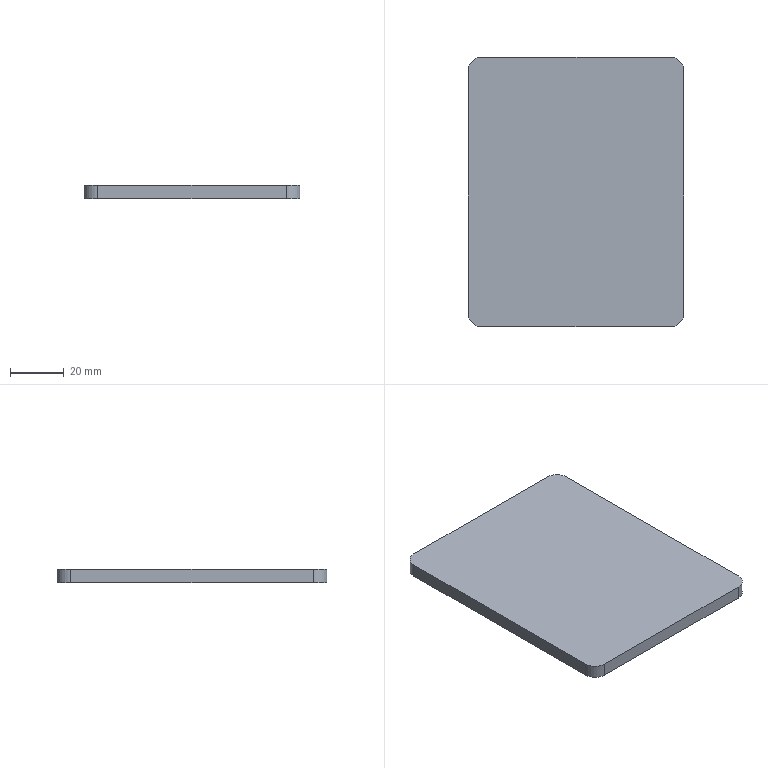Part | SolidWorks | features Extrusion 1, Fillet 1 | 1 solid | 10 faces | box 80 x 100 x 5 mm | volume 39893 mm3 | plane 6 | cylinder 4 | commonest cylinder face diameters 10 x4
STEP:
#1=CARTESIAN_POINT('',(0.,-5.,0.));
#2=VERTEX_POINT('',#1);
#3=CARTESIAN_POINT('',(0.,-95.,0.));
#4=VERTEX_POINT('',#3);
#5=CARTESIAN_POINT('',(0.,0.,0.));
#6=DIRECTION('',(0.,-1.,0.));
#7=VECTOR('',#6,1000.);
#8=LINE('',#5,#7);
#9=EDGE_CURVE('',#2,#4,#8,.T.);
#10=ORIENTED_EDGE('',*,*,#9,.T.);
#11=CARTESIAN_POINT('',(0.,-95.,5.));
#12=VERTEX_POINT('',#11);
#13=CARTESIAN_POINT('',(0.,-95.,5.));
#14=DIRECTION('',(0.,0.,1.));
#15=VECTOR('',#14,1000.);
#16=LINE('',#13,#15);
#17=EDGE_CURVE('',#4,#12,#16,.T.);
#18=ORIENTED_EDGE('',*,*,#17,.T.);
#19=CARTESIAN_POINT('',(0.,-5.,5.));
#20=VERTEX_POINT('',#19);
#21=CARTESIAN_POINT('',(0.,0.,5.));
#22=DIRECTION('',(0.,-1.,0.));
#23=VECTOR('',#22,1000.);
#24=LINE('',#21,#23);
#25=EDGE_CURVE('',#20,#12,#24,.T.);
#26=ORIENTED_EDGE('',*,*,#25,.F.);
#27=CARTESIAN_POINT('',(0.,-5.,5.));
#28=DIRECTION('',(0.,0.,-1.));
#29=VECTOR('',#28,1000.);
#30=LINE('',#27,#29);
#31=EDGE_CURVE('',#20,#2,#30,.T.);
#32=ORIENTED_EDGE('',*,*,#31,.T.);
#33=EDGE_LOOP('',(#10,#18,#26,#32));
#34=FACE_OUTER_BOUND('',#33,.T.);
#35=CARTESIAN_POINT('',(0.,0.,5.));
#36=DIRECTION('',(1.,0.,0.));
#37=DIRECTION('',(0.,1.,0.));
#38=AXIS2_PLACEMENT_3D('',#35,#36,#37);
#39=PLANE('',#38);
#40=ADVANCED_FACE('',(#34),#39,.F.);
#41=CARTESIAN_POINT('',(5.,-100.,0.));
#42=VERTEX_POINT('',#41);
#43=CARTESIAN_POINT('',(75.,-100.,0.));
#44=VERTEX_POINT('',#43);
#45=CARTESIAN_POINT('',(0.,-100.,0.));
#46=DIRECTION('',(1.,0.,0.));
#47=VECTOR('',#46,1000.);
#48=LINE('',#45,#47);
#49=EDGE_CURVE('',#42,#44,#48,.T.);
#50=ORIENTED_EDGE('',*,*,#49,.T.);
#51=CARTESIAN_POINT('',(75.,-100.,5.));
#52=VERTEX_POINT('',#51);
#53=CARTESIAN_POINT('',(75.,-100.,5.));
#54=DIRECTION('',(0.,0.,1.));
#55=VECTOR('',#54,1000.);
#56=LINE('',#53,#55);
#57=EDGE_CURVE('',#44,#52,#56,.T.);
#58=ORIENTED_EDGE('',*,*,#57,.T.);
#59=CARTESIAN_POINT('',(5.,-100.,5.));
#60=VERTEX_POINT('',#59);
#61=CARTESIAN_POINT('',(0.,-100.,5.));
#62=DIRECTION('',(1.,0.,0.));
#63=VECTOR('',#62,1000.);
#64=LINE('',#61,#63);
#65=EDGE_CURVE('',#60,#52,#64,.T.);
#66=ORIENTED_EDGE('',*,*,#65,.F.);
#67=CARTESIAN_POINT('',(5.,-100.,5.));
#68=DIRECTION('',(0.,0.,-1.));
#69=VECTOR('',#68,1000.);
#70=LINE('',#67,#69);
#71=EDGE_CURVE('',#60,#42,#70,.T.);
#72=ORIENTED_EDGE('',*,*,#71,.T.);
#73=EDGE_LOOP('',(#50,#58,#66,#72));
#74=FACE_OUTER_BOUND('',#73,.T.);
#75=CARTESIAN_POINT('',(0.,-100.,5.));
#76=DIRECTION('',(0.,1.,0.));
#77=DIRECTION('',(0.,0.,1.));
#78=AXIS2_PLACEMENT_3D('',#75,#76,#77);
#79=PLANE('',#78);
#80=ADVANCED_FACE('',(#74),#79,.F.);
#81=CARTESIAN_POINT('',(80.,-95.,5.));
#82=VERTEX_POINT('',#81);
#83=CARTESIAN_POINT('',(80.,-5.,5.));
#84=VERTEX_POINT('',#83);
#85=CARTESIAN_POINT('',(80.,0.,5.));
#86=DIRECTION('',(0.,1.,0.));
#87=VECTOR('',#86,1000.);
#88=LINE('',#85,#87);
#89=EDGE_CURVE('',#82,#84,#88,.T.);
#90=ORIENTED_EDGE('',*,*,#89,.F.);
#91=CARTESIAN_POINT('',(80.,-95.,0.));
#92=VERTEX_POINT('',#91);
#93=CARTESIAN_POINT('',(80.,-95.,5.));
#94=DIRECTION('',(0.,0.,-1.));
#95=VECTOR('',#94,1000.);
#96=LINE('',#93,#95);
#97=EDGE_CURVE('',#82,#92,#96,.T.);
#98=ORIENTED_EDGE('',*,*,#97,.T.);
#99=CARTESIAN_POINT('',(80.,-5.,0.));
#100=VERTEX_POINT('',#99);
#101=CARTESIAN_POINT('',(80.,0.,0.));
#102=DIRECTION('',(0.,1.,0.));
#103=VECTOR('',#102,1000.);
#104=LINE('',#101,#103);
#105=EDGE_CURVE('',#92,#100,#104,.T.);
#106=ORIENTED_EDGE('',*,*,#105,.T.);
#107=CARTESIAN_POINT('',(80.,-5.,5.));
#108=DIRECTION('',(0.,0.,1.));
#109=VECTOR('',#108,1000.);
#110=LINE('',#107,#109);
#111=EDGE_CURVE('',#100,#84,#110,.T.);
#112=ORIENTED_EDGE('',*,*,#111,.T.);
#113=EDGE_LOOP('',(#90,#98,#106,#112));
#114=FACE_OUTER_BOUND('',#113,.T.);
#115=CARTESIAN_POINT('',(80.,0.,5.));
#116=DIRECTION('',(-1.,0.,0.));
#117=DIRECTION('',(0.,-1.,0.));
#118=AXIS2_PLACEMENT_3D('',#115,#116,#117);
#119=PLANE('',#118);
#120=ADVANCED_FACE('',(#114),#119,.F.);
#121=CARTESIAN_POINT('',(75.,0.,5.));
#122=VERTEX_POINT('',#121);
#123=CARTESIAN_POINT('',(5.,0.,5.));
#124=VERTEX_POINT('',#123);
#125=CARTESIAN_POINT('',(0.,0.,5.));
#126=DIRECTION('',(-1.,0.,0.));
#127=VECTOR('',#126,1000.);
#128=LINE('',#125,#127);
#129=EDGE_CURVE('',#122,#124,#128,.T.);
#130=ORIENTED_EDGE('',*,*,#129,.F.);
#131=CARTESIAN_POINT('',(75.,0.,0.));
#132=VERTEX_POINT('',#131);
#133=CARTESIAN_POINT('',(75.,0.,5.));
#134=DIRECTION('',(0.,0.,-1.));
#135=VECTOR('',#134,1000.);
#136=LINE('',#133,#135);
#137=EDGE_CURVE('',#122,#132,#136,.T.);
#138=ORIENTED_EDGE('',*,*,#137,.T.);
#139=CARTESIAN_POINT('',(5.,0.,0.));
#140=VERTEX_POINT('',#139);
#141=CARTESIAN_POINT('',(0.,0.,0.));
#142=DIRECTION('',(-1.,0.,0.));
#143=VECTOR('',#142,1000.);
#144=LINE('',#141,#143);
#145=EDGE_CURVE('',#132,#140,#144,.T.);
#146=ORIENTED_EDGE('',*,*,#145,.T.);
#147=CARTESIAN_POINT('',(5.,0.,5.));
#148=DIRECTION('',(0.,0.,1.));
#149=VECTOR('',#148,1000.);
#150=LINE('',#147,#149);
#151=EDGE_CURVE('',#140,#124,#150,.T.);
#152=ORIENTED_EDGE('',*,*,#151,.T.);
#153=EDGE_LOOP('',(#130,#138,#146,#152));
#154=FACE_OUTER_BOUND('',#153,.T.);
#155=CARTESIAN_POINT('',(0.,0.,5.));
#156=DIRECTION('',(0.,-1.,0.));
#157=DIRECTION('',(0.,0.,-1.));
#158=AXIS2_PLACEMENT_3D('',#155,#156,#157);
#159=PLANE('',#158);
#160=ADVANCED_FACE('',(#154),#159,.F.);
#161=ORIENTED_EDGE('',*,*,#65,.T.);
#162=CARTESIAN_POINT('',(75.,-95.,5.));
#163=DIRECTION('',(0.,0.,1.));
#164=DIRECTION('',(1.,0.,0.));
#165=AXIS2_PLACEMENT_3D('',#162,#163,#164);
#166=CIRCLE('',#165,5.);
#167=EDGE_CURVE('',#52,#82,#166,.T.);
#168=ORIENTED_EDGE('',*,*,#167,.T.);
#169=ORIENTED_EDGE('',*,*,#89,.T.);
#170=CARTESIAN_POINT('',(75.,-5.,5.));
#171=DIRECTION('',(0.,0.,1.));
#172=DIRECTION('',(1.,0.,0.));
#173=AXIS2_PLACEMENT_3D('',#170,#171,#172);
#174=CIRCLE('',#173,5.);
#175=EDGE_CURVE('',#84,#122,#174,.T.);
#176=ORIENTED_EDGE('',*,*,#175,.T.);
#177=ORIENTED_EDGE('',*,*,#129,.T.);
#178=CARTESIAN_POINT('',(5.,-5.,5.));
#179=DIRECTION('',(0.,0.,1.));
#180=DIRECTION('',(1.,0.,0.));
#181=AXIS2_PLACEMENT_3D('',#178,#179,#180);
#182=CIRCLE('',#181,5.);
#183=EDGE_CURVE('',#124,#20,#182,.T.);
#184=ORIENTED_EDGE('',*,*,#183,.T.);
#185=ORIENTED_EDGE('',*,*,#25,.T.);
#186=CARTESIAN_POINT('',(5.,-95.,5.));
#187=DIRECTION('',(0.,0.,1.));
#188=DIRECTION('',(1.,0.,0.));
#189=AXIS2_PLACEMENT_3D('',#186,#187,#188);
#190=CIRCLE('',#189,5.);
#191=EDGE_CURVE('',#12,#60,#190,.T.);
#192=ORIENTED_EDGE('',*,*,#191,.T.);
#193=EDGE_LOOP('',(#161,#168,#169,#176,#177,#184,#185,#192));
#194=FACE_OUTER_BOUND('',#193,.T.);
#195=CARTESIAN_POINT('',(0.,0.,5.));
#196=DIRECTION('',(0.,0.,1.));
#197=DIRECTION('',(1.,0.,0.));
#198=AXIS2_PLACEMENT_3D('',#195,#196,#197);
#199=PLANE('',#198);
#200=ADVANCED_FACE('',(#194),#199,.T.);
#201=ORIENTED_EDGE('',*,*,#105,.F.);
#202=CARTESIAN_POINT('',(75.,-95.,0.));
#203=DIRECTION('',(0.,0.,-1.));
#204=DIRECTION('',(1.,0.,0.));
#205=AXIS2_PLACEMENT_3D('',#202,#203,#204);
#206=CIRCLE('',#205,5.);
#207=EDGE_CURVE('',#92,#44,#206,.T.);
#208=ORIENTED_EDGE('',*,*,#207,.T.);
#209=ORIENTED_EDGE('',*,*,#49,.F.);
#210=CARTESIAN_POINT('',(5.,-95.,0.));
#211=DIRECTION('',(0.,0.,-1.));
#212=DIRECTION('',(1.,0.,0.));
#213=AXIS2_PLACEMENT_3D('',#210,#211,#212);
#214=CIRCLE('',#213,5.);
#215=EDGE_CURVE('',#42,#4,#214,.T.);
#216=ORIENTED_EDGE('',*,*,#215,.T.);
#217=ORIENTED_EDGE('',*,*,#9,.F.);
#218=CARTESIAN_POINT('',(5.,-5.,0.));
#219=DIRECTION('',(0.,0.,-1.));
#220=DIRECTION('',(1.,0.,0.));
#221=AXIS2_PLACEMENT_3D('',#218,#219,#220);
#222=CIRCLE('',#221,5.);
#223=EDGE_CURVE('',#2,#140,#222,.T.);
#224=ORIENTED_EDGE('',*,*,#223,.T.);
#225=ORIENTED_EDGE('',*,*,#145,.F.);
#226=CARTESIAN_POINT('',(75.,-5.,0.));
#227=DIRECTION('',(0.,0.,-1.));
#228=DIRECTION('',(1.,0.,0.));
#229=AXIS2_PLACEMENT_3D('',#226,#227,#228);
#230=CIRCLE('',#229,5.);
#231=EDGE_CURVE('',#132,#100,#230,.T.);
#232=ORIENTED_EDGE('',*,*,#231,.T.);
#233=EDGE_LOOP('',(#201,#208,#209,#216,#217,#224,#225,#232));
#234=FACE_OUTER_BOUND('',#233,.T.);
#235=CARTESIAN_POINT('',(0.,0.,0.));
#236=DIRECTION('',(0.,0.,1.));
#237=DIRECTION('',(1.,0.,0.));
#238=AXIS2_PLACEMENT_3D('',#235,#236,#237);
#239=PLANE('',#238);
#240=ADVANCED_FACE('',(#234),#239,.F.);
#241=ORIENTED_EDGE('',*,*,#167,.F.);
#242=ORIENTED_EDGE('',*,*,#57,.F.);
#243=ORIENTED_EDGE('',*,*,#207,.F.);
#244=ORIENTED_EDGE('',*,*,#97,.F.);
#245=EDGE_LOOP('',(#241,#242,#243,#244));
#246=FACE_OUTER_BOUND('',#245,.T.);
#247=CARTESIAN_POINT('',(75.,-95.,5.));
#248=DIRECTION('',(0.,0.,-1.));
#249=DIRECTION('',(-1.,0.,0.));
#250=AXIS2_PLACEMENT_3D('',#247,#248,#249);
#251=CYLINDRICAL_SURFACE('',#250,5.);
#252=ADVANCED_FACE('',(#246),#251,.T.);
#253=ORIENTED_EDGE('',*,*,#191,.F.);
#254=ORIENTED_EDGE('',*,*,#17,.F.);
#255=ORIENTED_EDGE('',*,*,#215,.F.);
#256=ORIENTED_EDGE('',*,*,#71,.F.);
#257=EDGE_LOOP('',(#253,#254,#255,#256));
#258=FACE_OUTER_BOUND('',#257,.T.);
#259=CARTESIAN_POINT('',(5.,-95.,5.));
#260=DIRECTION('',(0.,0.,-1.));
#261=DIRECTION('',(-1.,0.,0.));
#262=AXIS2_PLACEMENT_3D('',#259,#260,#261);
#263=CYLINDRICAL_SURFACE('',#262,5.);
#264=ADVANCED_FACE('',(#258),#263,.T.);
#265=ORIENTED_EDGE('',*,*,#175,.F.);
#266=ORIENTED_EDGE('',*,*,#111,.F.);
#267=ORIENTED_EDGE('',*,*,#231,.F.);
#268=ORIENTED_EDGE('',*,*,#137,.F.);
#269=EDGE_LOOP('',(#265,#266,#267,#268));
#270=FACE_OUTER_BOUND('',#269,.T.);
#271=CARTESIAN_POINT('',(75.,-5.,5.));
#272=DIRECTION('',(0.,0.,-1.));
#273=DIRECTION('',(-1.,0.,0.));
#274=AXIS2_PLACEMENT_3D('',#271,#272,#273);
#275=CYLINDRICAL_SURFACE('',#274,5.);
#276=ADVANCED_FACE('',(#270),#275,.T.);
#277=ORIENTED_EDGE('',*,*,#183,.F.);
#278=ORIENTED_EDGE('',*,*,#151,.F.);
#279=ORIENTED_EDGE('',*,*,#223,.F.);
#280=ORIENTED_EDGE('',*,*,#31,.F.);
#281=EDGE_LOOP('',(#277,#278,#279,#280));
#282=FACE_OUTER_BOUND('',#281,.T.);
#283=CARTESIAN_POINT('',(5.,-5.,5.));
#284=DIRECTION('',(0.,0.,-1.));
#285=DIRECTION('',(-1.,0.,0.));
#286=AXIS2_PLACEMENT_3D('',#283,#284,#285);
#287=CYLINDRICAL_SURFACE('',#286,5.);
#288=ADVANCED_FACE('',(#282),#287,.T.);
#289=CLOSED_SHELL('',(#40,#80,#120,#160,#200,#240,#252,#264,#276,#288));
#290=MANIFOLD_SOLID_BREP('',#289);
#291=CARTESIAN_POINT('',(0.,0.,0.));
#292=DIRECTION('',(0.,0.,1.));
#293=DIRECTION('',(1.,0.,0.));
#294=AXIS2_PLACEMENT_3D('',#291,#292,#293);
#295=(LENGTH_UNIT()NAMED_UNIT(*)SI_UNIT(.MILLI.,.METRE.));
#296=UNCERTAINTY_MEASURE_WITH_UNIT(LENGTH_MEASURE(0.00001),#295,'','');
#297=(NAMED_UNIT(*)PLANE_ANGLE_UNIT()SI_UNIT($,.RADIAN.));
#298=(NAMED_UNIT(*)SI_UNIT($,.STERADIAN.)SOLID_ANGLE_UNIT());
#299=(GEOMETRIC_REPRESENTATION_CONTEXT(3)GLOBAL_UNCERTAINTY_ASSIGNED_CONTEXT((#296))GLOBAL_UNIT_ASSIGNED_CONTEXT((#295,#297,#298))REPRESENTATION_CONTEXT('',''));
#300=ADVANCED_BREP_SHAPE_REPRESENTATION('',(#290,#294),#299);